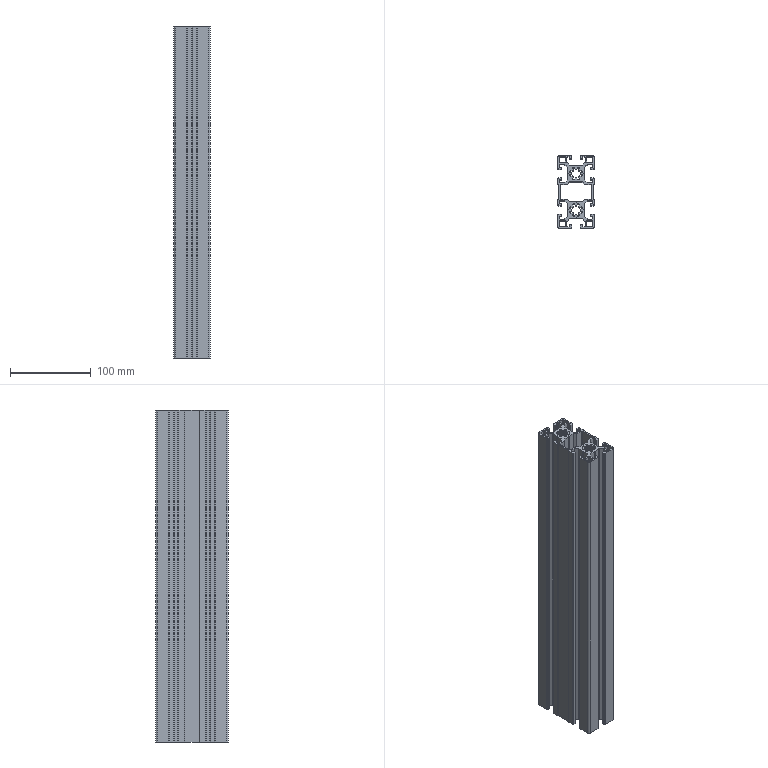Part | STEP file | PN_0026 | 1 solid | 468 faces | box 45 x 90 x 410 mm | volume 533346 mm3 | cylinder 262 | plane 206 | commonest cylinder face diameters 1 x116 0.6 x56 2 x40 10.2 x18 16 x16 0.4 x12